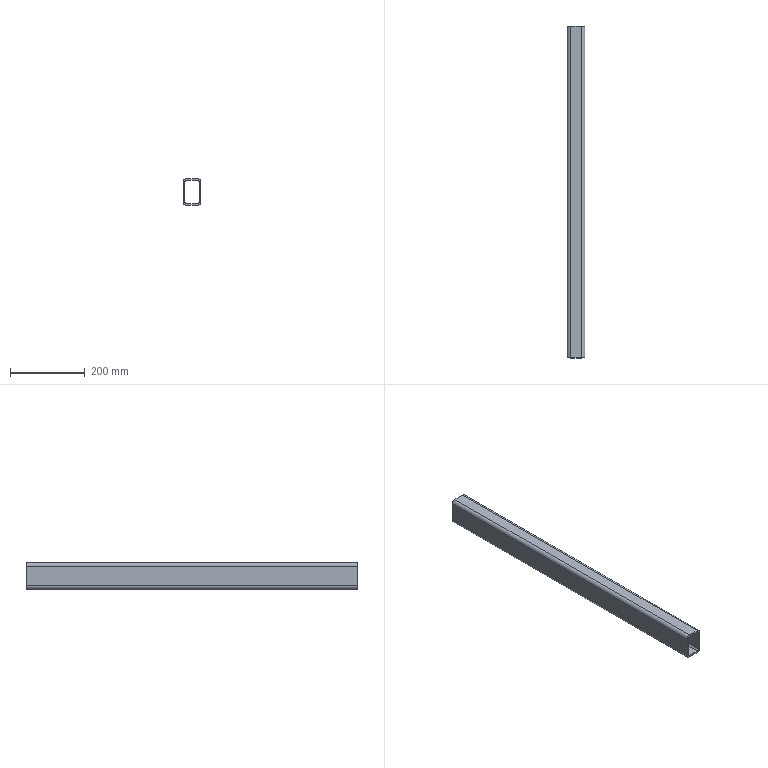Part | NX | 1 solid | 18 faces | box 48 x 887.916 x 72 mm | volume 888366 mm3 | plane 10 | cylinder 8 | commonest cylinder face diameters 9.6 x4 19.2 x4
STEP:
#1=CARTESIAN_POINT('',(268.674,131.097,634.353));
#2=VERTEX_POINT('',#1);
#3=CARTESIAN_POINT('',(278.274,131.097,643.953));
#4=VERTEX_POINT('',#3);
#5=CARTESIAN_POINT('',(278.274,131.097,634.353));
#6=DIRECTION('',(0.,1.,0.));
#7=DIRECTION('',(0.,0.,-1.));
#8=AXIS2_PLACEMENT_3D('',#5,#6,#7);
#9=CIRCLE('',#8,9.6);
#10=EDGE_CURVE('',#2,#4,#9,.T.);
#11=ORIENTED_EDGE('',*,*,#10,.F.);
#12=CARTESIAN_POINT('',(268.674,-756.819,634.353));
#13=VERTEX_POINT('',#12);
#14=CARTESIAN_POINT('',(268.674,-756.819,634.353));
#15=DIRECTION('',(0.,1.,0.));
#16=VECTOR('',#15,1.);
#17=LINE('',#14,#16);
#18=EDGE_CURVE('',#13,#2,#17,.T.);
#19=ORIENTED_EDGE('',*,*,#18,.F.);
#20=CARTESIAN_POINT('',(278.274,-756.819,643.953));
#21=VERTEX_POINT('',#20);
#22=CARTESIAN_POINT('',(278.274,-756.819,634.353));
#23=DIRECTION('',(0.,1.,0.));
#24=DIRECTION('',(0.,0.,-1.));
#25=AXIS2_PLACEMENT_3D('',#22,#23,#24);
#26=CIRCLE('',#25,9.6);
#27=EDGE_CURVE('',#13,#21,#26,.T.);
#28=ORIENTED_EDGE('',*,*,#27,.T.);
#29=CARTESIAN_POINT('',(278.274,-756.819,643.953));
#30=DIRECTION('',(0.,1.,0.));
#31=VECTOR('',#30,1.);
#32=LINE('',#29,#31);
#33=EDGE_CURVE('',#21,#4,#32,.T.);
#34=ORIENTED_EDGE('',*,*,#33,.T.);
#35=EDGE_LOOP('',(#11,#19,#28,#34));
#36=FACE_OUTER_BOUND('',#35,.T.);
#37=CARTESIAN_POINT('',(278.274,-756.819,634.353));
#38=DIRECTION('',(0.,1.,0.));
#39=DIRECTION('',(0.,0.,1.));
#40=AXIS2_PLACEMENT_3D('',#37,#38,#39);
#41=CYLINDRICAL_SURFACE('',#40,9.6);
#42=ADVANCED_FACE('',(#36),#41,.T.);
#43=CARTESIAN_POINT('',(307.074,131.097,643.953));
#44=VERTEX_POINT('',#43);
#45=CARTESIAN_POINT('',(278.274,131.097,643.953));
#46=DIRECTION('',(1.,0.,0.));
#47=VECTOR('',#46,1.);
#48=LINE('',#45,#47);
#49=EDGE_CURVE('',#4,#44,#48,.T.);
#50=ORIENTED_EDGE('',*,*,#49,.F.);
#51=ORIENTED_EDGE('',*,*,#33,.F.);
#52=CARTESIAN_POINT('',(307.074,-756.819,643.953));
#53=VERTEX_POINT('',#52);
#54=CARTESIAN_POINT('',(278.274,-756.819,643.953));
#55=DIRECTION('',(1.,0.,0.));
#56=VECTOR('',#55,1.);
#57=LINE('',#54,#56);
#58=EDGE_CURVE('',#21,#53,#57,.T.);
#59=ORIENTED_EDGE('',*,*,#58,.T.);
#60=CARTESIAN_POINT('',(307.074,-756.819,643.953));
#61=DIRECTION('',(0.,1.,0.));
#62=VECTOR('',#61,1.);
#63=LINE('',#60,#62);
#64=EDGE_CURVE('',#53,#44,#63,.T.);
#65=ORIENTED_EDGE('',*,*,#64,.T.);
#66=EDGE_LOOP('',(#50,#51,#59,#65));
#67=FACE_OUTER_BOUND('',#66,.T.);
#68=CARTESIAN_POINT('',(278.274,-756.819,643.953));
#69=DIRECTION('',(0.,0.,-1.));
#70=DIRECTION('',(1.,0.,0.));
#71=AXIS2_PLACEMENT_3D('',#68,#69,#70);
#72=PLANE('',#71);
#73=ADVANCED_FACE('',(#67),#72,.F.);
#74=CARTESIAN_POINT('',(316.674,131.097,634.353));
#75=VERTEX_POINT('',#74);
#76=CARTESIAN_POINT('',(307.074,131.097,634.353));
#77=DIRECTION('',(0.,1.,0.));
#78=DIRECTION('',(0.,0.,-1.));
#79=AXIS2_PLACEMENT_3D('',#76,#77,#78);
#80=CIRCLE('',#79,9.6);
#81=EDGE_CURVE('',#44,#75,#80,.T.);
#82=ORIENTED_EDGE('',*,*,#81,.F.);
#83=ORIENTED_EDGE('',*,*,#64,.F.);
#84=CARTESIAN_POINT('',(316.674,-756.819,634.353));
#85=VERTEX_POINT('',#84);
#86=CARTESIAN_POINT('',(307.074,-756.819,634.353));
#87=DIRECTION('',(0.,1.,0.));
#88=DIRECTION('',(0.,0.,-1.));
#89=AXIS2_PLACEMENT_3D('',#86,#87,#88);
#90=CIRCLE('',#89,9.6);
#91=EDGE_CURVE('',#53,#85,#90,.T.);
#92=ORIENTED_EDGE('',*,*,#91,.T.);
#93=CARTESIAN_POINT('',(316.674,-756.819,634.353));
#94=DIRECTION('',(0.,1.,0.));
#95=VECTOR('',#94,1.);
#96=LINE('',#93,#95);
#97=EDGE_CURVE('',#85,#75,#96,.T.);
#98=ORIENTED_EDGE('',*,*,#97,.T.);
#99=EDGE_LOOP('',(#82,#83,#92,#98));
#100=FACE_OUTER_BOUND('',#99,.T.);
#101=CARTESIAN_POINT('',(307.074,-756.819,634.353));
#102=DIRECTION('',(0.,1.,0.));
#103=DIRECTION('',(0.,0.,1.));
#104=AXIS2_PLACEMENT_3D('',#101,#102,#103);
#105=CYLINDRICAL_SURFACE('',#104,9.6);
#106=ADVANCED_FACE('',(#100),#105,.T.);
#107=CARTESIAN_POINT('',(316.674,131.097,581.553));
#108=VERTEX_POINT('',#107);
#109=CARTESIAN_POINT('',(316.674,131.097,581.553));
#110=DIRECTION('',(0.,0.,-1.));
#111=VECTOR('',#110,1.);
#112=LINE('',#109,#111);
#113=EDGE_CURVE('',#75,#108,#112,.T.);
#114=ORIENTED_EDGE('',*,*,#113,.F.);
#115=ORIENTED_EDGE('',*,*,#97,.F.);
#116=CARTESIAN_POINT('',(316.674,-756.819,581.553));
#117=VERTEX_POINT('',#116);
#118=CARTESIAN_POINT('',(316.674,-756.819,581.553));
#119=DIRECTION('',(0.,0.,-1.));
#120=VECTOR('',#119,1.);
#121=LINE('',#118,#120);
#122=EDGE_CURVE('',#85,#117,#121,.T.);
#123=ORIENTED_EDGE('',*,*,#122,.T.);
#124=CARTESIAN_POINT('',(316.674,-756.819,581.553));
#125=DIRECTION('',(0.,1.,0.));
#126=VECTOR('',#125,1.);
#127=LINE('',#124,#126);
#128=EDGE_CURVE('',#117,#108,#127,.T.);
#129=ORIENTED_EDGE('',*,*,#128,.T.);
#130=EDGE_LOOP('',(#114,#115,#123,#129));
#131=FACE_OUTER_BOUND('',#130,.T.);
#132=CARTESIAN_POINT('',(316.674,-756.819,581.553));
#133=DIRECTION('',(-1.,0.,0.));
#134=DIRECTION('',(0.,0.,-1.));
#135=AXIS2_PLACEMENT_3D('',#132,#133,#134);
#136=PLANE('',#135);
#137=ADVANCED_FACE('',(#131),#136,.F.);
#138=CARTESIAN_POINT('',(307.074,131.097,571.953));
#139=VERTEX_POINT('',#138);
#140=CARTESIAN_POINT('',(307.074,131.097,581.553));
#141=DIRECTION('',(0.,1.,0.));
#142=DIRECTION('',(0.,0.,-1.));
#143=AXIS2_PLACEMENT_3D('',#140,#141,#142);
#144=CIRCLE('',#143,9.6);
#145=EDGE_CURVE('',#108,#139,#144,.T.);
#146=ORIENTED_EDGE('',*,*,#145,.F.);
#147=ORIENTED_EDGE('',*,*,#128,.F.);
#148=CARTESIAN_POINT('',(307.074,-756.819,571.953));
#149=VERTEX_POINT('',#148);
#150=CARTESIAN_POINT('',(307.074,-756.819,581.553));
#151=DIRECTION('',(0.,1.,0.));
#152=DIRECTION('',(0.,0.,-1.));
#153=AXIS2_PLACEMENT_3D('',#150,#151,#152);
#154=CIRCLE('',#153,9.6);
#155=EDGE_CURVE('',#117,#149,#154,.T.);
#156=ORIENTED_EDGE('',*,*,#155,.T.);
#157=CARTESIAN_POINT('',(307.074,-756.819,571.953));
#158=DIRECTION('',(0.,1.,0.));
#159=VECTOR('',#158,1.);
#160=LINE('',#157,#159);
#161=EDGE_CURVE('',#149,#139,#160,.T.);
#162=ORIENTED_EDGE('',*,*,#161,.T.);
#163=EDGE_LOOP('',(#146,#147,#156,#162));
#164=FACE_OUTER_BOUND('',#163,.T.);
#165=CARTESIAN_POINT('',(307.074,-756.819,581.553));
#166=DIRECTION('',(0.,1.,0.));
#167=DIRECTION('',(0.,0.,1.));
#168=AXIS2_PLACEMENT_3D('',#165,#166,#167);
#169=CYLINDRICAL_SURFACE('',#168,9.6);
#170=ADVANCED_FACE('',(#164),#169,.T.);
#171=CARTESIAN_POINT('',(278.274,131.097,571.953));
#172=VERTEX_POINT('',#171);
#173=CARTESIAN_POINT('',(307.074,131.097,571.953));
#174=DIRECTION('',(-1.,0.,0.));
#175=VECTOR('',#174,1.);
#176=LINE('',#173,#175);
#177=EDGE_CURVE('',#139,#172,#176,.T.);
#178=ORIENTED_EDGE('',*,*,#177,.F.);
#179=ORIENTED_EDGE('',*,*,#161,.F.);
#180=CARTESIAN_POINT('',(278.274,-756.819,571.953));
#181=VERTEX_POINT('',#180);
#182=CARTESIAN_POINT('',(307.074,-756.819,571.953));
#183=DIRECTION('',(-1.,0.,0.));
#184=VECTOR('',#183,1.);
#185=LINE('',#182,#184);
#186=EDGE_CURVE('',#149,#181,#185,.T.);
#187=ORIENTED_EDGE('',*,*,#186,.T.);
#188=CARTESIAN_POINT('',(278.274,-756.819,571.953));
#189=DIRECTION('',(0.,1.,0.));
#190=VECTOR('',#189,1.);
#191=LINE('',#188,#190);
#192=EDGE_CURVE('',#181,#172,#191,.T.);
#193=ORIENTED_EDGE('',*,*,#192,.T.);
#194=EDGE_LOOP('',(#178,#179,#187,#193));
#195=FACE_OUTER_BOUND('',#194,.T.);
#196=CARTESIAN_POINT('',(307.074,-756.819,571.953));
#197=DIRECTION('',(0.,0.,1.));
#198=DIRECTION('',(-1.,0.,0.));
#199=AXIS2_PLACEMENT_3D('',#196,#197,#198);
#200=PLANE('',#199);
#201=ADVANCED_FACE('',(#195),#200,.F.);
#202=CARTESIAN_POINT('',(268.674,131.097,581.553));
#203=VERTEX_POINT('',#202);
#204=CARTESIAN_POINT('',(278.274,131.097,581.553));
#205=DIRECTION('',(0.,1.,0.));
#206=DIRECTION('',(0.,0.,-1.));
#207=AXIS2_PLACEMENT_3D('',#204,#205,#206);
#208=CIRCLE('',#207,9.6);
#209=EDGE_CURVE('',#172,#203,#208,.T.);
#210=ORIENTED_EDGE('',*,*,#209,.F.);
#211=ORIENTED_EDGE('',*,*,#192,.F.);
#212=CARTESIAN_POINT('',(268.674,-756.819,581.553));
#213=VERTEX_POINT('',#212);
#214=CARTESIAN_POINT('',(278.274,-756.819,581.553));
#215=DIRECTION('',(0.,1.,0.));
#216=DIRECTION('',(0.,0.,-1.));
#217=AXIS2_PLACEMENT_3D('',#214,#215,#216);
#218=CIRCLE('',#217,9.6);
#219=EDGE_CURVE('',#181,#213,#218,.T.);
#220=ORIENTED_EDGE('',*,*,#219,.T.);
#221=CARTESIAN_POINT('',(268.674,-756.819,581.553));
#222=DIRECTION('',(0.,1.,0.));
#223=VECTOR('',#222,1.);
#224=LINE('',#221,#223);
#225=EDGE_CURVE('',#213,#203,#224,.T.);
#226=ORIENTED_EDGE('',*,*,#225,.T.);
#227=EDGE_LOOP('',(#210,#211,#220,#226));
#228=FACE_OUTER_BOUND('',#227,.T.);
#229=CARTESIAN_POINT('',(278.274,-756.819,581.553));
#230=DIRECTION('',(0.,1.,0.));
#231=DIRECTION('',(0.,0.,1.));
#232=AXIS2_PLACEMENT_3D('',#229,#230,#231);
#233=CYLINDRICAL_SURFACE('',#232,9.6);
#234=ADVANCED_FACE('',(#228),#233,.T.);
#235=CARTESIAN_POINT('',(307.074,131.097,639.153));
#236=VERTEX_POINT('',#235);
#237=CARTESIAN_POINT('',(311.874,131.097,634.353));
#238=VERTEX_POINT('',#237);
#239=CARTESIAN_POINT('',(307.074,131.097,634.353));
#240=DIRECTION('',(0.,1.,0.));
#241=DIRECTION('',(0.,0.,-1.));
#242=AXIS2_PLACEMENT_3D('',#239,#240,#241);
#243=CIRCLE('',#242,4.8);
#244=EDGE_CURVE('',#236,#238,#243,.T.);
#245=ORIENTED_EDGE('',*,*,#244,.T.);
#246=CARTESIAN_POINT('',(311.874,-756.819,634.353));
#247=VERTEX_POINT('',#246);
#248=CARTESIAN_POINT('',(311.874,-756.819,634.353));
#249=DIRECTION('',(0.,1.,0.));
#250=VECTOR('',#249,1.);
#251=LINE('',#248,#250);
#252=EDGE_CURVE('',#247,#238,#251,.T.);
#253=ORIENTED_EDGE('',*,*,#252,.F.);
#254=CARTESIAN_POINT('',(307.074,-756.819,639.153));
#255=VERTEX_POINT('',#254);
#256=CARTESIAN_POINT('',(307.074,-756.819,634.353));
#257=DIRECTION('',(0.,1.,0.));
#258=DIRECTION('',(0.,0.,-1.));
#259=AXIS2_PLACEMENT_3D('',#256,#257,#258);
#260=CIRCLE('',#259,4.8);
#261=EDGE_CURVE('',#255,#247,#260,.T.);
#262=ORIENTED_EDGE('',*,*,#261,.F.);
#263=CARTESIAN_POINT('',(307.074,-756.819,639.153));
#264=DIRECTION('',(0.,1.,0.));
#265=VECTOR('',#264,1.);
#266=LINE('',#263,#265);
#267=EDGE_CURVE('',#255,#236,#266,.T.);
#268=ORIENTED_EDGE('',*,*,#267,.T.);
#269=EDGE_LOOP('',(#245,#253,#262,#268));
#270=FACE_OUTER_BOUND('',#269,.T.);
#271=CARTESIAN_POINT('',(307.074,-756.819,634.353));
#272=DIRECTION('',(0.,1.,0.));
#273=DIRECTION('',(0.,0.,1.));
#274=AXIS2_PLACEMENT_3D('',#271,#272,#273);
#275=CYLINDRICAL_SURFACE('',#274,4.8);
#276=ADVANCED_FACE('',(#270),#275,.F.);
#277=CARTESIAN_POINT('',(278.274,131.097,639.153));
#278=VERTEX_POINT('',#277);
#279=CARTESIAN_POINT('',(278.274,131.097,639.153));
#280=DIRECTION('',(1.,0.,0.));
#281=VECTOR('',#280,1.);
#282=LINE('',#279,#281);
#283=EDGE_CURVE('',#278,#236,#282,.T.);
#284=ORIENTED_EDGE('',*,*,#283,.T.);
#285=ORIENTED_EDGE('',*,*,#267,.F.);
#286=CARTESIAN_POINT('',(278.274,-756.819,639.153));
#287=VERTEX_POINT('',#286);
#288=CARTESIAN_POINT('',(278.274,-756.819,639.153));
#289=DIRECTION('',(1.,0.,0.));
#290=VECTOR('',#289,1.);
#291=LINE('',#288,#290);
#292=EDGE_CURVE('',#287,#255,#291,.T.);
#293=ORIENTED_EDGE('',*,*,#292,.F.);
#294=CARTESIAN_POINT('',(278.274,-756.819,639.153));
#295=DIRECTION('',(0.,1.,0.));
#296=VECTOR('',#295,1.);
#297=LINE('',#294,#296);
#298=EDGE_CURVE('',#287,#278,#297,.T.);
#299=ORIENTED_EDGE('',*,*,#298,.T.);
#300=EDGE_LOOP('',(#284,#285,#293,#299));
#301=FACE_OUTER_BOUND('',#300,.T.);
#302=CARTESIAN_POINT('',(278.274,-756.819,639.153));
#303=DIRECTION('',(0.,0.,-1.));
#304=DIRECTION('',(1.,0.,0.));
#305=AXIS2_PLACEMENT_3D('',#302,#303,#304);
#306=PLANE('',#305);
#307=ADVANCED_FACE('',(#301),#306,.T.);
#308=CARTESIAN_POINT('',(273.474,131.097,634.353));
#309=VERTEX_POINT('',#308);
#310=CARTESIAN_POINT('',(278.274,131.097,634.353));
#311=DIRECTION('',(0.,1.,0.));
#312=DIRECTION('',(0.,0.,-1.));
#313=AXIS2_PLACEMENT_3D('',#310,#311,#312);
#314=CIRCLE('',#313,4.8);
#315=EDGE_CURVE('',#309,#278,#314,.T.);
#316=ORIENTED_EDGE('',*,*,#315,.T.);
#317=ORIENTED_EDGE('',*,*,#298,.F.);
#318=CARTESIAN_POINT('',(273.474,-756.819,634.353));
#319=VERTEX_POINT('',#318);
#320=CARTESIAN_POINT('',(278.274,-756.819,634.353));
#321=DIRECTION('',(0.,1.,0.));
#322=DIRECTION('',(0.,0.,-1.));
#323=AXIS2_PLACEMENT_3D('',#320,#321,#322);
#324=CIRCLE('',#323,4.8);
#325=EDGE_CURVE('',#319,#287,#324,.T.);
#326=ORIENTED_EDGE('',*,*,#325,.F.);
#327=CARTESIAN_POINT('',(273.474,-756.819,634.353));
#328=DIRECTION('',(0.,1.,0.));
#329=VECTOR('',#328,1.);
#330=LINE('',#327,#329);
#331=EDGE_CURVE('',#319,#309,#330,.T.);
#332=ORIENTED_EDGE('',*,*,#331,.T.);
#333=EDGE_LOOP('',(#316,#317,#326,#332));
#334=FACE_OUTER_BOUND('',#333,.T.);
#335=CARTESIAN_POINT('',(278.274,-756.819,634.353));
#336=DIRECTION('',(0.,1.,0.));
#337=DIRECTION('',(0.,0.,1.));
#338=AXIS2_PLACEMENT_3D('',#335,#336,#337);
#339=CYLINDRICAL_SURFACE('',#338,4.8);
#340=ADVANCED_FACE('',(#334),#339,.F.);
#341=CARTESIAN_POINT('',(273.474,131.097,581.553));
#342=VERTEX_POINT('',#341);
#343=CARTESIAN_POINT('',(273.474,131.097,634.353));
#344=DIRECTION('',(0.,0.,1.));
#345=VECTOR('',#344,1.);
#346=LINE('',#343,#345);
#347=EDGE_CURVE('',#342,#309,#346,.T.);
#348=ORIENTED_EDGE('',*,*,#347,.T.);
#349=ORIENTED_EDGE('',*,*,#331,.F.);
#350=CARTESIAN_POINT('',(273.474,-756.819,581.553));
#351=VERTEX_POINT('',#350);
#352=CARTESIAN_POINT('',(273.474,-756.819,634.353));
#353=DIRECTION('',(0.,0.,1.));
#354=VECTOR('',#353,1.);
#355=LINE('',#352,#354);
#356=EDGE_CURVE('',#351,#319,#355,.T.);
#357=ORIENTED_EDGE('',*,*,#356,.F.);
#358=CARTESIAN_POINT('',(273.474,-756.819,581.553));
#359=DIRECTION('',(0.,1.,0.));
#360=VECTOR('',#359,1.);
#361=LINE('',#358,#360);
#362=EDGE_CURVE('',#351,#342,#361,.T.);
#363=ORIENTED_EDGE('',*,*,#362,.T.);
#364=EDGE_LOOP('',(#348,#349,#357,#363));
#365=FACE_OUTER_BOUND('',#364,.T.);
#366=CARTESIAN_POINT('',(273.474,-756.819,634.353));
#367=DIRECTION('',(1.,0.,0.));
#368=DIRECTION('',(0.,0.,1.));
#369=AXIS2_PLACEMENT_3D('',#366,#367,#368);
#370=PLANE('',#369);
#371=ADVANCED_FACE('',(#365),#370,.T.);
#372=CARTESIAN_POINT('',(278.274,131.097,576.753));
#373=VERTEX_POINT('',#372);
#374=CARTESIAN_POINT('',(278.274,131.097,581.553));
#375=DIRECTION('',(0.,1.,0.));
#376=DIRECTION('',(0.,0.,-1.));
#377=AXIS2_PLACEMENT_3D('',#374,#375,#376);
#378=CIRCLE('',#377,4.8);
#379=EDGE_CURVE('',#373,#342,#378,.T.);
#380=ORIENTED_EDGE('',*,*,#379,.T.);
#381=ORIENTED_EDGE('',*,*,#362,.F.);
#382=CARTESIAN_POINT('',(278.274,-756.819,576.753));
#383=VERTEX_POINT('',#382);
#384=CARTESIAN_POINT('',(278.274,-756.819,581.553));
#385=DIRECTION('',(0.,1.,0.));
#386=DIRECTION('',(0.,0.,-1.));
#387=AXIS2_PLACEMENT_3D('',#384,#385,#386);
#388=CIRCLE('',#387,4.8);
#389=EDGE_CURVE('',#383,#351,#388,.T.);
#390=ORIENTED_EDGE('',*,*,#389,.F.);
#391=CARTESIAN_POINT('',(278.274,-756.819,576.753));
#392=DIRECTION('',(0.,1.,0.));
#393=VECTOR('',#392,1.);
#394=LINE('',#391,#393);
#395=EDGE_CURVE('',#383,#373,#394,.T.);
#396=ORIENTED_EDGE('',*,*,#395,.T.);
#397=EDGE_LOOP('',(#380,#381,#390,#396));
#398=FACE_OUTER_BOUND('',#397,.T.);
#399=CARTESIAN_POINT('',(278.274,-756.819,581.553));
#400=DIRECTION('',(0.,1.,0.));
#401=DIRECTION('',(0.,0.,1.));
#402=AXIS2_PLACEMENT_3D('',#399,#400,#401);
#403=CYLINDRICAL_SURFACE('',#402,4.8);
#404=ADVANCED_FACE('',(#398),#403,.F.);
#405=CARTESIAN_POINT('',(307.074,131.097,576.753));
#406=VERTEX_POINT('',#405);
#407=CARTESIAN_POINT('',(307.074,131.097,576.753));
#408=DIRECTION('',(-1.,0.,0.));
#409=VECTOR('',#408,1.);
#410=LINE('',#407,#409);
#411=EDGE_CURVE('',#406,#373,#410,.T.);
#412=ORIENTED_EDGE('',*,*,#411,.T.);
#413=ORIENTED_EDGE('',*,*,#395,.F.);
#414=CARTESIAN_POINT('',(307.074,-756.819,576.753));
#415=VERTEX_POINT('',#414);
#416=CARTESIAN_POINT('',(307.074,-756.819,576.753));
#417=DIRECTION('',(-1.,0.,0.));
#418=VECTOR('',#417,1.);
#419=LINE('',#416,#418);
#420=EDGE_CURVE('',#415,#383,#419,.T.);
#421=ORIENTED_EDGE('',*,*,#420,.F.);
#422=CARTESIAN_POINT('',(307.074,-756.819,576.753));
#423=DIRECTION('',(0.,1.,0.));
#424=VECTOR('',#423,1.);
#425=LINE('',#422,#424);
#426=EDGE_CURVE('',#415,#406,#425,.T.);
#427=ORIENTED_EDGE('',*,*,#426,.T.);
#428=EDGE_LOOP('',(#412,#413,#421,#427));
#429=FACE_OUTER_BOUND('',#428,.T.);
#430=CARTESIAN_POINT('',(307.074,-756.819,576.753));
#431=DIRECTION('',(0.,0.,1.));
#432=DIRECTION('',(-1.,0.,0.));
#433=AXIS2_PLACEMENT_3D('',#430,#431,#432);
#434=PLANE('',#433);
#435=ADVANCED_FACE('',(#429),#434,.T.);
#436=CARTESIAN_POINT('',(311.874,131.097,581.553));
#437=VERTEX_POINT('',#436);
#438=CARTESIAN_POINT('',(307.074,131.097,581.553));
#439=DIRECTION('',(0.,1.,0.));
#440=DIRECTION('',(0.,0.,-1.));
#441=AXIS2_PLACEMENT_3D('',#438,#439,#440);
#442=CIRCLE('',#441,4.8);
#443=EDGE_CURVE('',#437,#406,#442,.T.);
#444=ORIENTED_EDGE('',*,*,#443,.T.);
#445=ORIENTED_EDGE('',*,*,#426,.F.);
#446=CARTESIAN_POINT('',(311.874,-756.819,581.553));
#447=VERTEX_POINT('',#446);
#448=CARTESIAN_POINT('',(307.074,-756.819,581.553));
#449=DIRECTION('',(0.,1.,0.));
#450=DIRECTION('',(0.,0.,-1.));
#451=AXIS2_PLACEMENT_3D('',#448,#449,#450);
#452=CIRCLE('',#451,4.8);
#453=EDGE_CURVE('',#447,#415,#452,.T.);
#454=ORIENTED_EDGE('',*,*,#453,.F.);
#455=CARTESIAN_POINT('',(311.874,-756.819,581.553));
#456=DIRECTION('',(0.,1.,0.));
#457=VECTOR('',#456,1.);
#458=LINE('',#455,#457);
#459=EDGE_CURVE('',#447,#437,#458,.T.);
#460=ORIENTED_EDGE('',*,*,#459,.T.);
#461=EDGE_LOOP('',(#444,#445,#454,#460));
#462=FACE_OUTER_BOUND('',#461,.T.);
#463=CARTESIAN_POINT('',(307.074,-756.819,581.553));
#464=DIRECTION('',(0.,1.,0.));
#465=DIRECTION('',(0.,0.,1.));
#466=AXIS2_PLACEMENT_3D('',#463,#464,#465);
#467=CYLINDRICAL_SURFACE('',#466,4.8);
#468=ADVANCED_FACE('',(#462),#467,.F.);
#469=CARTESIAN_POINT('',(311.874,131.097,581.553));
#470=DIRECTION('',(0.,0.,-1.));
#471=VECTOR('',#470,1.);
#472=LINE('',#469,#471);
#473=EDGE_CURVE('',#238,#437,#472,.T.);
#474=ORIENTED_EDGE('',*,*,#473,.T.);
#475=ORIENTED_EDGE('',*,*,#459,.F.);
#476=CARTESIAN_POINT('',(311.874,-756.819,581.553));
#477=DIRECTION('',(0.,0.,-1.));
#478=VECTOR('',#477,1.);
#479=LINE('',#476,#478);
#480=EDGE_CURVE('',#247,#447,#479,.T.);
#481=ORIENTED_EDGE('',*,*,#480,.F.);
#482=ORIENTED_EDGE('',*,*,#252,.T.);
#483=EDGE_LOOP('',(#474,#475,#481,#482));
#484=FACE_OUTER_BOUND('',#483,.T.);
#485=CARTESIAN_POINT('',(311.874,-756.819,581.553));
#486=DIRECTION('',(-1.,0.,0.));
#487=DIRECTION('',(0.,0.,-1.));
#488=AXIS2_PLACEMENT_3D('',#485,#486,#487);
#489=PLANE('',#488);
#490=ADVANCED_FACE('',(#484),#489,.T.);
#491=CARTESIAN_POINT('',(268.674,131.097,634.353));
#492=DIRECTION('',(0.,0.,1.));
#493=VECTOR('',#492,1.);
#494=LINE('',#491,#493);
#495=EDGE_CURVE('',#203,#2,#494,.T.);
#496=ORIENTED_EDGE('',*,*,#495,.F.);
#497=ORIENTED_EDGE('',*,*,#225,.F.);
#498=CARTESIAN_POINT('',(268.674,-756.819,634.353));
#499=DIRECTION('',(0.,0.,1.));
#500=VECTOR('',#499,1.);
#501=LINE('',#498,#500);
#502=EDGE_CURVE('',#213,#13,#501,.T.);
#503=ORIENTED_EDGE('',*,*,#502,.T.);
#504=ORIENTED_EDGE('',*,*,#18,.T.);
#505=EDGE_LOOP('',(#496,#497,#503,#504));
#506=FACE_OUTER_BOUND('',#505,.T.);
#507=CARTESIAN_POINT('',(268.674,-756.819,634.353));
#508=DIRECTION('',(1.,0.,0.));
#509=DIRECTION('',(0.,0.,1.));
#510=AXIS2_PLACEMENT_3D('',#507,#508,#509);
#511=PLANE('',#510);
#512=ADVANCED_FACE('',(#506),#511,.F.);
#513=ORIENTED_EDGE('',*,*,#261,.T.);
#514=ORIENTED_EDGE('',*,*,#480,.T.);
#515=ORIENTED_EDGE('',*,*,#453,.T.);
#516=ORIENTED_EDGE('',*,*,#420,.T.);
#517=ORIENTED_EDGE('',*,*,#389,.T.);
#518=ORIENTED_EDGE('',*,*,#356,.T.);
#519=ORIENTED_EDGE('',*,*,#325,.T.);
#520=ORIENTED_EDGE('',*,*,#292,.T.);
#521=EDGE_LOOP('',(#513,#514,#515,#516,#517,#518,#519,#520));
#522=FACE_BOUND('',#521,.T.);
#523=ORIENTED_EDGE('',*,*,#27,.F.);
#524=ORIENTED_EDGE('',*,*,#502,.F.);
#525=ORIENTED_EDGE('',*,*,#219,.F.);
#526=ORIENTED_EDGE('',*,*,#186,.F.);
#527=ORIENTED_EDGE('',*,*,#155,.F.);
#528=ORIENTED_EDGE('',*,*,#122,.F.);
#529=ORIENTED_EDGE('',*,*,#91,.F.);
#530=ORIENTED_EDGE('',*,*,#58,.F.);
#531=EDGE_LOOP('',(#523,#524,#525,#526,#527,#528,#529,#530));
#532=FACE_BOUND('',#531,.T.);
#533=CARTESIAN_POINT('',(278.274,-756.819,634.353));
#534=DIRECTION('',(0.,-1.,0.));
#535=DIRECTION('',(0.,0.,-1.));
#536=AXIS2_PLACEMENT_3D('',#533,#534,#535);
#537=PLANE('',#536);
#538=ADVANCED_FACE('',(#522,#532),#537,.T.);
#539=ORIENTED_EDGE('',*,*,#244,.F.);
#540=ORIENTED_EDGE('',*,*,#283,.F.);
#541=ORIENTED_EDGE('',*,*,#315,.F.);
#542=ORIENTED_EDGE('',*,*,#347,.F.);
#543=ORIENTED_EDGE('',*,*,#379,.F.);
#544=ORIENTED_EDGE('',*,*,#411,.F.);
#545=ORIENTED_EDGE('',*,*,#443,.F.);
#546=ORIENTED_EDGE('',*,*,#473,.F.);
#547=EDGE_LOOP('',(#539,#540,#541,#542,#543,#544,#545,#546));
#548=FACE_BOUND('',#547,.T.);
#549=ORIENTED_EDGE('',*,*,#10,.T.);
#550=ORIENTED_EDGE('',*,*,#49,.T.);
#551=ORIENTED_EDGE('',*,*,#81,.T.);
#552=ORIENTED_EDGE('',*,*,#113,.T.);
#553=ORIENTED_EDGE('',*,*,#145,.T.);
#554=ORIENTED_EDGE('',*,*,#177,.T.);
#555=ORIENTED_EDGE('',*,*,#209,.T.);
#556=ORIENTED_EDGE('',*,*,#495,.T.);
#557=EDGE_LOOP('',(#549,#550,#551,#552,#553,#554,#555,#556));
#558=FACE_BOUND('',#557,.T.);
#559=CARTESIAN_POINT('',(278.274,131.097,634.353));
#560=DIRECTION('',(0.,-1.,0.));
#561=DIRECTION('',(0.,0.,-1.));
#562=AXIS2_PLACEMENT_3D('',#559,#560,#561);
#563=PLANE('',#562);
#564=ADVANCED_FACE('',(#548,#558),#563,.F.);
#565=CLOSED_SHELL('',(#42,#73,#106,#137,#170,#201,#234,#276,#307,#340,#371,#404,#435,#468,#490,#512,#538,#564));
#566=MANIFOLD_SOLID_BREP('',#565);
#567=(LENGTH_UNIT()NAMED_UNIT(*)SI_UNIT(.MILLI.,.METRE.));
#568=UNCERTAINTY_MEASURE_WITH_UNIT(LENGTH_MEASURE(0.00002),#567,'','');
#569=(NAMED_UNIT(*)PLANE_ANGLE_UNIT()SI_UNIT($,.RADIAN.));
#570=PLANE_ANGLE_MEASURE_WITH_UNIT(PLANE_ANGLE_MEASURE(0.01745),#569);
#571=DIMENSIONAL_EXPONENTS(0.,0.,0.,0.,0.,0.,0.);
#572=(CONVERSION_BASED_UNIT('DEGREE',#570)NAMED_UNIT(#571)PLANE_ANGLE_UNIT());
#573=(NAMED_UNIT(*)SI_UNIT($,.STERADIAN.)SOLID_ANGLE_UNIT());
#574=(GEOMETRIC_REPRESENTATION_CONTEXT(3)GLOBAL_UNCERTAINTY_ASSIGNED_CONTEXT((#568))GLOBAL_UNIT_ASSIGNED_CONTEXT((#567,#572,#573))REPRESENTATION_CONTEXT('',''));
#575=ADVANCED_BREP_SHAPE_REPRESENTATION('',(#566),#574);